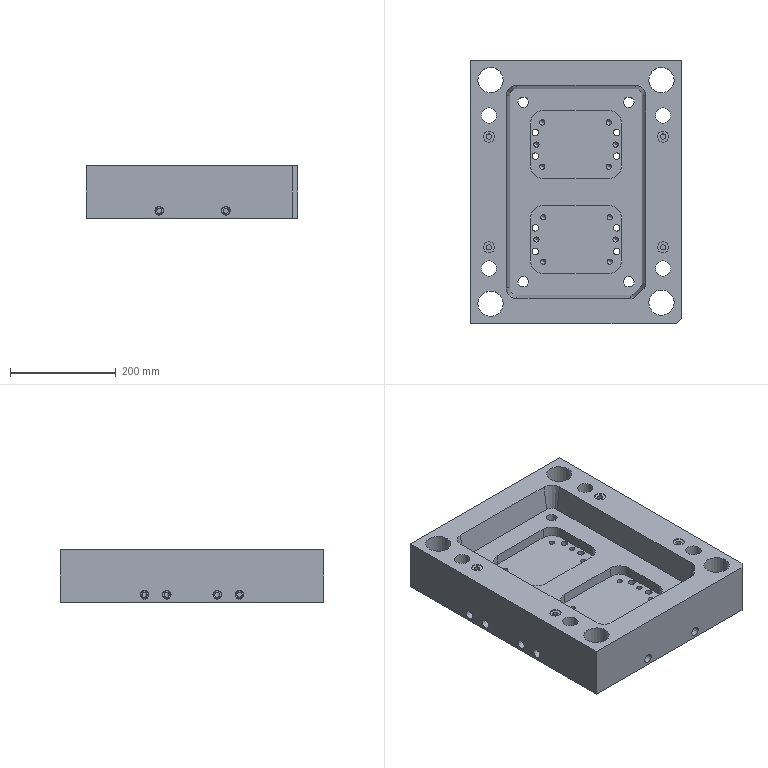Part | STEP file | SL2-MOLD_id754_xmt_txt | 1 solid | 229 faces | box 400 x 500 x 99 mm | volume 12276978 mm3 | cylinder 110 | plane 90 | cone 29 | commonest cylinder face diameters 10 x52 12.5 x8 19 x8 49.326 x8 16 x6 20 x4